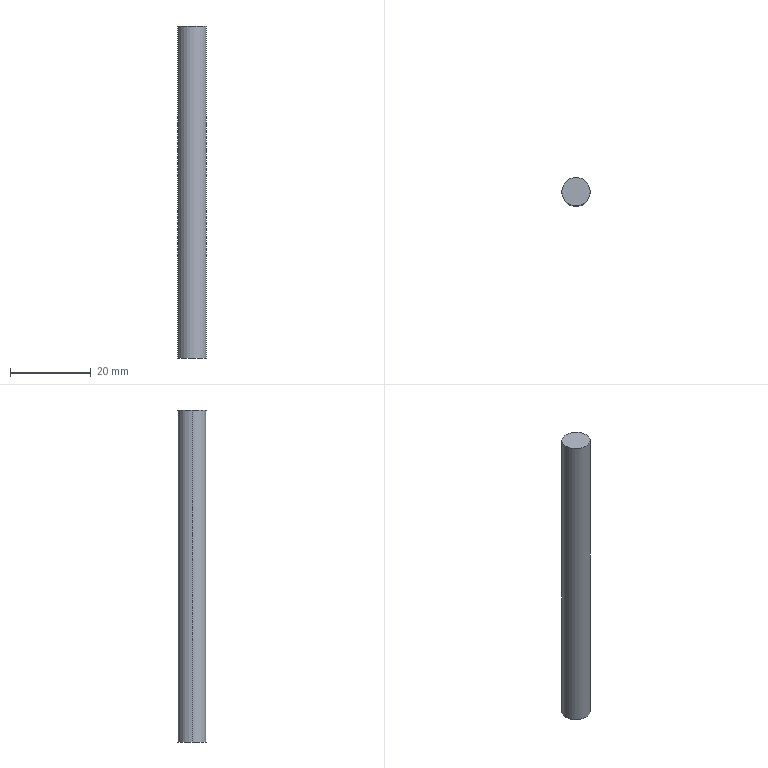Part | STEP file | _AKQ01-G-Z-6279A-002-ZZ | 1 solid | 4 faces | box 7 x 7 x 82 mm | volume 3156 mm3 | cylinder 2 | plane 2 | commonest cylinder face diameters 7 x2
STEP:
#1=CARTESIAN_POINT('',(0.,0.,0.));
#2=DIRECTION('',(0.,0.,1.));
#3=DIRECTION('',(1.,0.,0.));
#4=AXIS2_PLACEMENT_3D('',#1,#2,#3);
#5=CARTESIAN_POINT('',(3.5,0.,-41.));
#6=VERTEX_POINT('',#5);
#7=CARTESIAN_POINT('',(-3.5,0.,-41.));
#8=VERTEX_POINT('',#7);
#9=CARTESIAN_POINT('',(0.,0.,-41.));
#10=DIRECTION('',(0.,0.,1.));
#11=DIRECTION('',(1.,0.,0.));
#12=AXIS2_PLACEMENT_3D('',#9,#10,#11);
#13=CIRCLE('',#12,3.5);
#14=CARTESIAN_POINT('',(0.,0.,41.));
#15=DIRECTION('',(0.,0.,1.));
#16=DIRECTION('',(1.,0.,0.));
#17=AXIS2_PLACEMENT_3D('',#14,#15,#16);
#18=CYLINDRICAL_SURFACE('',#17,3.5);
#19=CARTESIAN_POINT('',(0.,-82.));
#20=DIRECTION('',(1.,0.));
#21=VECTOR('',#20,1.);
#22=LINE('',#19,#21);
#23=(GEOMETRIC_REPRESENTATION_CONTEXT(2)PARAMETRIC_REPRESENTATION_CONTEXT()REPRESENTATION_CONTEXT('',''));
#24=DEFINITIONAL_REPRESENTATION('',(#22),#23);
#25=PCURVE('',#18,#24);
#26=CARTESIAN_POINT('',(0.,0.,-41.));
#27=DIRECTION('',(0.,0.,1.));
#28=DIRECTION('',(1.,0.,0.));
#29=AXIS2_PLACEMENT_3D('',#26,#27,#28);
#30=PLANE('',#29);
#31=CARTESIAN_POINT('',(0.,0.));
#32=DIRECTION('',(1.,0.));
#33=AXIS2_PLACEMENT_2D('',#31,#32);
#34=CIRCLE('',#33,3.5);
#35=(GEOMETRIC_REPRESENTATION_CONTEXT(2)PARAMETRIC_REPRESENTATION_CONTEXT()REPRESENTATION_CONTEXT('',''));
#36=DEFINITIONAL_REPRESENTATION('',(#34),#35);
#37=PCURVE('',#30,#36);
#38=SURFACE_CURVE('',#13,(#25,#37),.PCURVE_S1.);
#39=EDGE_CURVE('',#6,#8,#38,.T.);
#40=ORIENTED_EDGE('',*,*,#39,.T.);
#41=CARTESIAN_POINT('',(-3.5,0.,41.));
#42=VERTEX_POINT('',#41);
#43=CARTESIAN_POINT('',(-3.5,0.,41.));
#44=DIRECTION('',(0.,0.,1.));
#45=VECTOR('',#44,1.);
#46=LINE('',#43,#45);
#47=CARTESIAN_POINT('',(3.142,0.));
#48=DIRECTION('',(0.,1.));
#49=VECTOR('',#48,1.);
#50=LINE('',#47,#49);
#51=(GEOMETRIC_REPRESENTATION_CONTEXT(2)PARAMETRIC_REPRESENTATION_CONTEXT()REPRESENTATION_CONTEXT('',''));
#52=DEFINITIONAL_REPRESENTATION('',(#50),#51);
#53=PCURVE('',#18,#52);
#54=CARTESIAN_POINT('',(0.,0.,41.));
#55=DIRECTION('',(0.,0.,1.));
#56=DIRECTION('',(1.,0.,0.));
#57=AXIS2_PLACEMENT_3D('',#54,#55,#56);
#58=CYLINDRICAL_SURFACE('',#57,3.5);
#59=CARTESIAN_POINT('',(3.142,0.));
#60=DIRECTION('',(0.,1.));
#61=VECTOR('',#60,1.);
#62=LINE('',#59,#61);
#63=(GEOMETRIC_REPRESENTATION_CONTEXT(2)PARAMETRIC_REPRESENTATION_CONTEXT()REPRESENTATION_CONTEXT('',''));
#64=DEFINITIONAL_REPRESENTATION('',(#62),#63);
#65=PCURVE('',#58,#64);
#66=SURFACE_CURVE('',#46,(#53,#65),.PCURVE_S1.);
#67=EDGE_CURVE('',#8,#42,#66,.T.);
#68=ORIENTED_EDGE('',*,*,#67,.T.);
#69=CARTESIAN_POINT('',(3.5,0.,41.));
#70=VERTEX_POINT('',#69);
#71=CARTESIAN_POINT('',(0.,0.,41.));
#72=DIRECTION('',(0.,0.,-1.));
#73=DIRECTION('',(1.,0.,0.));
#74=AXIS2_PLACEMENT_3D('',#71,#72,#73);
#75=CIRCLE('',#74,3.5);
#76=CARTESIAN_POINT('',(6.283,0.));
#77=DIRECTION('',(-1.,0.));
#78=VECTOR('',#77,1.);
#79=LINE('',#76,#78);
#80=(GEOMETRIC_REPRESENTATION_CONTEXT(2)PARAMETRIC_REPRESENTATION_CONTEXT()REPRESENTATION_CONTEXT('',''));
#81=DEFINITIONAL_REPRESENTATION('',(#79),#80);
#82=PCURVE('',#18,#81);
#83=CARTESIAN_POINT('',(0.,0.,41.));
#84=DIRECTION('',(0.,0.,1.));
#85=DIRECTION('',(1.,0.,0.));
#86=AXIS2_PLACEMENT_3D('',#83,#84,#85);
#87=PLANE('',#86);
#88=CARTESIAN_POINT('',(3.5,0.));
#89=CARTESIAN_POINT('',(3.5,-6.062));
#90=CARTESIAN_POINT('',(-1.75,-3.031));
#91=CARTESIAN_POINT('',(-7.,0.));
#92=CARTESIAN_POINT('',(-1.75,3.031));
#93=CARTESIAN_POINT('',(3.5,6.062));
#94=CARTESIAN_POINT('',(3.5,0.));
#95=(BOUNDED_CURVE()B_SPLINE_CURVE(2,(#88,#89,#90,#91,#92,#93,#94),.UNSPECIFIED.,.T.,.F.)B_SPLINE_CURVE_WITH_KNOTS((1,2,2,2,2,1),(-2.094,0.,2.094,4.189,6.283,8.378),.UNSPECIFIED.)CURVE()GEOMETRIC_REPRESENTATION_ITEM()RATIONAL_B_SPLINE_CURVE((1.,0.5,1.,0.5,1.,0.5,1.))REPRESENTATION_ITEM(''));
#96=(GEOMETRIC_REPRESENTATION_CONTEXT(2)PARAMETRIC_REPRESENTATION_CONTEXT()REPRESENTATION_CONTEXT('',''));
#97=DEFINITIONAL_REPRESENTATION('',(#95),#96);
#98=PCURVE('',#87,#97);
#99=SURFACE_CURVE('',#75,(#82,#98),.PCURVE_S1.);
#100=EDGE_CURVE('',#42,#70,#99,.T.);
#101=ORIENTED_EDGE('',*,*,#100,.T.);
#102=CARTESIAN_POINT('',(3.5,0.,41.));
#103=DIRECTION('',(0.,0.,1.));
#104=VECTOR('',#103,1.);
#105=LINE('',#102,#104);
#106=CARTESIAN_POINT('',(0.,0.));
#107=DIRECTION('',(0.,1.));
#108=VECTOR('',#107,1.);
#109=LINE('',#106,#108);
#110=(GEOMETRIC_REPRESENTATION_CONTEXT(2)PARAMETRIC_REPRESENTATION_CONTEXT()REPRESENTATION_CONTEXT('',''));
#111=DEFINITIONAL_REPRESENTATION('',(#109),#110);
#112=PCURVE('',#18,#111);
#113=CARTESIAN_POINT('',(6.283,0.));
#114=DIRECTION('',(0.,1.));
#115=VECTOR('',#114,1.);
#116=LINE('',#113,#115);
#117=(GEOMETRIC_REPRESENTATION_CONTEXT(2)PARAMETRIC_REPRESENTATION_CONTEXT()REPRESENTATION_CONTEXT('',''));
#118=DEFINITIONAL_REPRESENTATION('',(#116),#117);
#119=PCURVE('',#58,#118);
#120=SURFACE_CURVE('',#105,(#112,#119),.PCURVE_S1.);
#121=EDGE_CURVE('',#6,#70,#120,.T.);
#122=ORIENTED_EDGE('',*,*,#121,.F.);
#123=EDGE_LOOP('',(#40,#68,#101,#122));
#124=FACE_BOUND('',#123,.T.);
#125=ADVANCED_FACE('',(#124),#18,.T.);
#126=ORIENTED_EDGE('',*,*,#67,.F.);
#127=CARTESIAN_POINT('',(0.,0.,-41.));
#128=DIRECTION('',(0.,0.,1.));
#129=DIRECTION('',(1.,0.,0.));
#130=AXIS2_PLACEMENT_3D('',#127,#128,#129);
#131=CIRCLE('',#130,3.5);
#132=CARTESIAN_POINT('',(0.,-82.));
#133=DIRECTION('',(1.,0.));
#134=VECTOR('',#133,1.);
#135=LINE('',#132,#134);
#136=(GEOMETRIC_REPRESENTATION_CONTEXT(2)PARAMETRIC_REPRESENTATION_CONTEXT()REPRESENTATION_CONTEXT('',''));
#137=DEFINITIONAL_REPRESENTATION('',(#135),#136);
#138=PCURVE('',#58,#137);
#139=CARTESIAN_POINT('',(0.,0.));
#140=DIRECTION('',(1.,0.));
#141=AXIS2_PLACEMENT_2D('',#139,#140);
#142=CIRCLE('',#141,3.5);
#143=(GEOMETRIC_REPRESENTATION_CONTEXT(2)PARAMETRIC_REPRESENTATION_CONTEXT()REPRESENTATION_CONTEXT('',''));
#144=DEFINITIONAL_REPRESENTATION('',(#142),#143);
#145=PCURVE('',#30,#144);
#146=SURFACE_CURVE('',#131,(#138,#145),.PCURVE_S1.);
#147=EDGE_CURVE('',#8,#6,#146,.T.);
#148=ORIENTED_EDGE('',*,*,#147,.T.);
#149=ORIENTED_EDGE('',*,*,#121,.T.);
#150=CARTESIAN_POINT('',(0.,0.,41.));
#151=DIRECTION('',(0.,0.,-1.));
#152=DIRECTION('',(1.,0.,0.));
#153=AXIS2_PLACEMENT_3D('',#150,#151,#152);
#154=CIRCLE('',#153,3.5);
#155=CARTESIAN_POINT('',(6.283,0.));
#156=DIRECTION('',(-1.,0.));
#157=VECTOR('',#156,1.);
#158=LINE('',#155,#157);
#159=(GEOMETRIC_REPRESENTATION_CONTEXT(2)PARAMETRIC_REPRESENTATION_CONTEXT()REPRESENTATION_CONTEXT('',''));
#160=DEFINITIONAL_REPRESENTATION('',(#158),#159);
#161=PCURVE('',#58,#160);
#162=CARTESIAN_POINT('',(3.5,0.));
#163=CARTESIAN_POINT('',(3.5,-6.062));
#164=CARTESIAN_POINT('',(-1.75,-3.031));
#165=CARTESIAN_POINT('',(-7.,0.));
#166=CARTESIAN_POINT('',(-1.75,3.031));
#167=CARTESIAN_POINT('',(3.5,6.062));
#168=CARTESIAN_POINT('',(3.5,0.));
#169=(BOUNDED_CURVE()B_SPLINE_CURVE(2,(#162,#163,#164,#165,#166,#167,#168),.UNSPECIFIED.,.T.,.F.)B_SPLINE_CURVE_WITH_KNOTS((1,2,2,2,2,1),(-2.094,0.,2.094,4.189,6.283,8.378),.UNSPECIFIED.)CURVE()GEOMETRIC_REPRESENTATION_ITEM()RATIONAL_B_SPLINE_CURVE((1.,0.5,1.,0.5,1.,0.5,1.))REPRESENTATION_ITEM(''));
#170=(GEOMETRIC_REPRESENTATION_CONTEXT(2)PARAMETRIC_REPRESENTATION_CONTEXT()REPRESENTATION_CONTEXT('',''));
#171=DEFINITIONAL_REPRESENTATION('',(#169),#170);
#172=PCURVE('',#87,#171);
#173=SURFACE_CURVE('',#154,(#161,#172),.PCURVE_S1.);
#174=EDGE_CURVE('',#70,#42,#173,.T.);
#175=ORIENTED_EDGE('',*,*,#174,.T.);
#176=EDGE_LOOP('',(#126,#148,#149,#175));
#177=FACE_BOUND('',#176,.T.);
#178=ADVANCED_FACE('',(#177),#58,.T.);
#179=ORIENTED_EDGE('',*,*,#39,.F.);
#180=ORIENTED_EDGE('',*,*,#147,.F.);
#181=EDGE_LOOP('',(#179,#180));
#182=FACE_BOUND('',#181,.T.);
#183=ADVANCED_FACE('',(#182),#30,.F.);
#184=ORIENTED_EDGE('',*,*,#174,.F.);
#185=ORIENTED_EDGE('',*,*,#100,.F.);
#186=EDGE_LOOP('',(#184,#185));
#187=FACE_BOUND('',#186,.T.);
#188=ADVANCED_FACE('',(#187),#87,.T.);
#189=CLOSED_SHELL('',(#125,#178,#183,#188));
#190=MANIFOLD_SOLID_BREP('',#189);
#191=(LENGTH_UNIT()NAMED_UNIT(*)SI_UNIT(.MILLI.,.METRE.));
#192=UNCERTAINTY_MEASURE_WITH_UNIT(LENGTH_MEASURE(0.0000001),#191,'','');
#193=(NAMED_UNIT(*)PLANE_ANGLE_UNIT()SI_UNIT($,.RADIAN.));
#194=(NAMED_UNIT(*)SI_UNIT($,.STERADIAN.)SOLID_ANGLE_UNIT());
#195=(GEOMETRIC_REPRESENTATION_CONTEXT(3)GLOBAL_UNCERTAINTY_ASSIGNED_CONTEXT((#192))GLOBAL_UNIT_ASSIGNED_CONTEXT((#191,#193,#194))REPRESENTATION_CONTEXT('',''));
#196=ADVANCED_BREP_SHAPE_REPRESENTATION('',(#4,#190),#195);